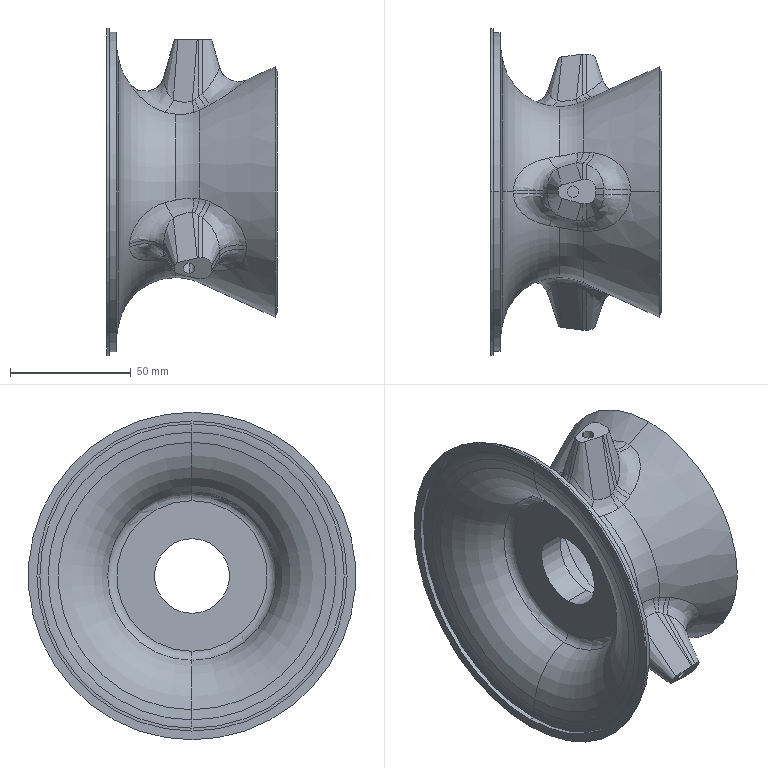Part | STEP file | Completa.sldasm-Part-60_Valor predeterminado | 1 solid | 151 faces | box 70.584 x 135.805 x 135.805 mm | volume 140836 mm3 | spline 42 | plane 37 | cylinder 28 | cone 28 | torus 16 | commonest cylinder face diameters 3.22 x10 4.891 x6 31 x2 55 x2 74.256 x2 128.613 x2